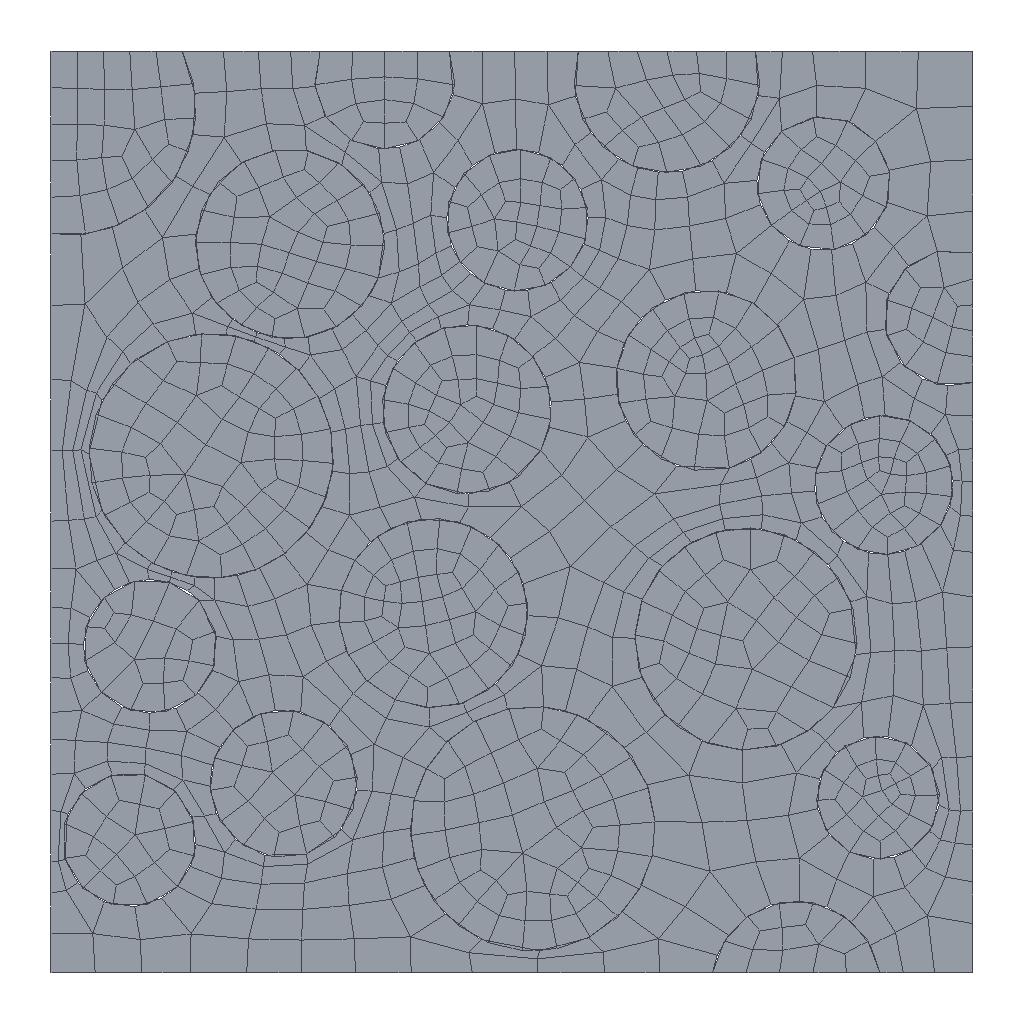Simulation study | abaqus
Set-up summary:
category,name,step,type,value,unit,region
solver,abaqus
solver,version,,,Abaqus/Standard 2020
units,not stated in the deck,,not stated
analysis,deck,,transient,transient
load_step,Step-1,Step-1,transient
load_step,requested,,,1
mesh,nodes,,,1351
mesh,elements,,,1025
element_type,CPS4R,,plane,1025
load,load commands in deck,,count,1
bc,support commands in deck,,count,5
material,JITI,,in results
material,KELI,,in results
check,setup vs results,,match,"per instance, exact: element labels, types and connectivity; labels of the nodes the elements use; coordinates of those nodes at SINGLE_PRECISION in 2 of 2 instance(s)"
Abaqus input file, long lists of numbers shortened:
*Heading
** Job name: Job-1 Model name: Model-1
** Generated by: Abaqus/CAE 2020
*Preprint, echo=NO, model=NO, history=NO, contact=NO
**
** PARTS
**
*Part, name=Part-2
*Node
      1, 0.0624,  0.1327
      2,  0.4349,          -1.
** (737 more lines like these left out)
*Element, type=CPS4R
 1, 312,  30,  31, 313
 2, 294, 312, 313, 303
** (572 more lines like these left out)
*Nset, nset=Set-2, generate
   1,  739,    1
*Elset, elset=Set-2, generate
   1,  574,    1
** Section: keli
*Solid Section, elset=Set-2, material=keli
,
*End Part
**
*Part, name=Part-3
*Node
      1,  0.7855,  0.6173
      2,  0.8594,  0.534
** (610 more lines like these left out)
*Element, type=CPS4R
  1, 230,   1, 231, 523
  2, 231,   2, 232, 523
** (449 more lines like these left out)
*Nset, nset=Set-3, generate
   1,  612,    1
*Elset, elset=Set-3, generate
   1,  451,    1
** Section: jiti
*Solid Section, elset=Set-3, material=jiti
,
*End Part
**
**
** ASSEMBLY
**
*Assembly, name=Assembly
**
*Instance, name=Part-2-1, part=Part-2
*End Instance
**
*Instance, name=Part-3-1, part=Part-3
*End Instance
**
*Node
      1, 0.004062,           1.,           0.
*Nset, nset=Set-1, instance=Part-2-1
  2,  3, 41, 42, 43, 44
*Nset, nset=Set-1, instance=Part-3-1
 163, 164, 165, 166, 179, 181, 195, 199, 211, 222, 229, 443, 445, 480, 481, 516
 522,
*Elset, elset=Set-1, instance=Part-2-1
 39, 40, 42, 44, 49
*Elset, elset=Set-1, instance=Part-3-1
 316, 317, 320, 321, 342, 343, 374, 378, 386, 387, 407, 437, 438, 447, 448
*Nset, nset=Set-3
 1,
*Nset, nset=Set-4, instance=Part-3-1
   9,  11,  21,  54,  55,  68, 145, 146, 149, 239, 254, 255, 303, 323, 424, 429
*Elset, elset=Set-4, instance=Part-3-1
  11,  15,  30,  31,  32, 100, 101, 130, 131, 284, 285, 289, 291
*Nset, nset=Set-5
 1,
*Nset, nset=Set-6, instance=Part-2-1
  4,  5, 11, 12, 51, 52, 53, 54, 89, 90, 91, 92
*Nset, nset=Set-6, instance=Part-3-1
   3,   4,  11,  28,  29,  39,  53,  67,  78,  97, 119, 136, 160, 179, 186, 188
 200, 213, 214, 216, 217, 220, 223, 225, 228, 229, 233, 242, 266, 336, 365, 440
** (1 more lines like these left out)
*Elset, elset=Set-6, instance=Part-2-1
  52,  56,  57,  58,  59, 108, 110, 111, 113, 123
*Elset, elset=Set-6, instance=Part-3-1
   3,   4,  14,  15,  46,  47,  67,  97, 128, 146, 152, 194, 195, 232, 268, 311
 314, 342, 357, 365, 391, 418, 421, 422, 425, 426, 429, 433, 440, 442, 443, 446
** (1 more lines like these left out)
*Nset, nset=m_Set-2
 1,
*Elset, elset=_m_Surf-2_S1, internal, instance=Part-3-1
   1,   3,   4,   6,   9,  11,  13,  15,  18,  20,  23,  25,  26,  28,  29,  32
  33,  35,  38,  41,  43,  45,  47,  50,  52,  57,  61,  64,  66,  69,  76,  80
** (8 more lines like these left out)
*Elset, elset=_m_Surf-2_S2, internal, instance=Part-3-1
   2,   3,   5,   8,  10,  12,  14,  15,  17,  19,  22,  24,  27,  30,  31,  32
  34,  37,  40,  42,  44,  46,  47,  49,  51,  56,  60,  63,  65,  68,  73,  74
** (9 more lines like these left out)
*Elset, elset=_m_Surf-2_S3, internal, instance=Part-3-1
 231, 260, 284, 285, 320, 321, 327, 342, 377, 405, 418
*Elset, elset=_m_Surf-2_S4, internal, instance=Part-3-1
  67,  78,  92,  96, 127, 148, 149, 217, 219, 232, 245, 266, 293, 309, 312, 322
 333, 335, 343, 366, 373, 388, 439, 441, 443, 450
*Surface, type=ELEMENT, name=m_Surf-2
_m_Surf-2_S1, S1
_m_Surf-2_S2, S2
_m_Surf-2_S4, S4
_m_Surf-2_S3, S3
*Elset, elset=_s_Surf-1_S1, internal, instance=Part-3-1
  11,  32, 101, 131, 289, 291
*Elset, elset=_s_Surf-1_S2, internal, instance=Part-3-1
  15,  30,  31, 100, 130
*Elset, elset=_s_Surf-1_S3, internal, instance=Part-3-1
 284, 285
*Surface, type=ELEMENT, name=s_Surf-1
_s_Surf-1_S1, S1
_s_Surf-1_S2, S2
_s_Surf-1_S3, S3
*Elset, elset=_s_Surf-2_S2, internal, instance=Part-2-1
   1,   8,   9,  37,  39,  44,  49,  56,  72,  77,  90, 108, 115, 119, 123, 160
 170, 177, 178, 207, 213, 223, 224, 225, 226, 227, 236, 243, 244, 260, 261, 262
** (4 more lines like these left out)
*Elset, elset=_s_Surf-2_S1, internal, instance=Part-2-1
   7,  21,  29,  30,  33,  35,  39,  43,  47,  49,  56,  57,  63,  65,  71,  75
  78,  79,  84,  85,  88,  97,  99, 102, 108, 109, 110, 117, 136, 138, 139, 144
** (4 more lines like these left out)
*Elset, elset=_s_Surf-2_S4, internal, instance=Part-2-1
  12,  13,  14,  15,  17,  40,  42,  45,  54,  57,  58,  59,  62,  65,  66,  88
  91,  93,  96, 102, 104, 107, 110, 113, 118, 120, 137, 150, 152, 153, 159, 167
** (3 more lines like these left out)
*Elset, elset=_s_Surf-2_S3, internal, instance=Part-2-1
  19,  46,  48,  52,  53,  60,  66,  69,  70,  83,  86,  89,  90,  92, 100, 111
 116, 128, 130, 131, 134, 176, 184, 191, 198, 210, 228, 250, 266, 270, 277, 289
** (2 more lines like these left out)
*Surface, type=ELEMENT, name=s_Surf-2
_s_Surf-2_S2, S2
_s_Surf-2_S1, S1
_s_Surf-2_S4, S4
_s_Surf-2_S3, S3
** Constraint: Constraint-1
*Coupling, constraint name=Constraint-1, ref node=m_Set-2, surface=s_Surf-1
*Kinematic
*End Assembly
*Amplitude, name=Amp-1
             0.,              0.,              1.,              1.
**
** MATERIALS
**
*Material, name=jiti
*Density
 1.027e-09,
*Elastic
476., 0.49
*Material, name=keli
*Density
 1.78e-09,
*Elastic
324500., 0.14
**
** INTERACTION PROPERTIES
**
*Surface Interaction, name=IntProp-1
1.,
*Friction, slip tolerance=0.005
 0.2,
*Surface Behavior, pressure-overclosure=HARD
**
** INTERACTIONS
**
** Interaction: Int-1
*Contact Pair, interaction=IntProp-1, type=SURFACE TO SURFACE
s_Surf-2, m_Surf-2
** ----------------------------------------------------------------
**
** STEP: Step-1
**
*Step, name=Step-1, nlgeom=NO, inc=1000
*Dynamic
0.001,1.,1e-05
**
** BOUNDARY CONDITIONS
**
** Name: BC-1 Type: 对称/反对称/完全固定
*Boundary
Set-1, ENCASTRE
** Name: BC-2 Type: 位移/转角
*Boundary, amplitude=Amp-1
Set-5, 1, 1
Set-5, 2, 2, 0.005
Set-5, 6, 6
** Name: BC-3 Type: 位移/转角
*Boundary
Set-6, 1, 1
**
** OUTPUT REQUESTS
**
*Restart, write, frequency=0
**
** FIELD OUTPUT: F-Output-1
**
*Output, field, frequency=1
*Node Output
CF, RF, U, V
*Element Output, directions=YES
E, LE, MISES, PE, PEEQ, PEMAG, S
*Contact Output
CDISP, CSTRESS
**
** HISTORY OUTPUT: H-Output-1
**
*Output, history, variable=PRESELECT, frequency=1
*End Step
Results summary:
result,step,,completed,increments=32 time=1.0/1.0
result,analysis,,,transient
result,last_loadstep,,,1
result,primary field,,,U
result,reaction total,,FX,-0.0,model units
result,reaction total,,FY,0.0,model units
result,reaction total,,FZ,0.0,model units